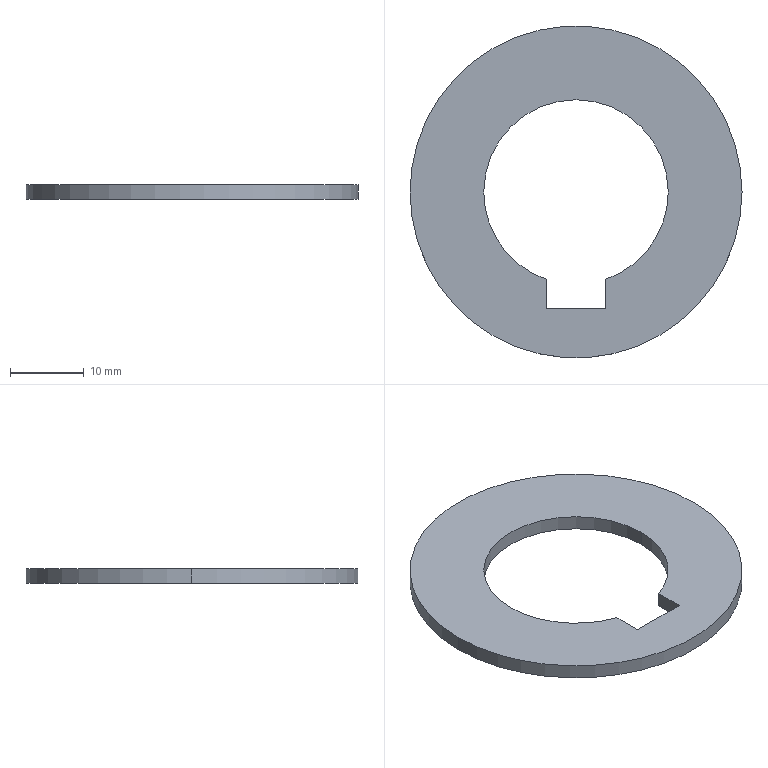Part | NX | 1 solid | 10 faces | box 45 x 45 x 2 mm | volume 2143 mm3 | plane 5 | cylinder 5 | commonest cylinder face diameters 25 x3 45 x2
STEP:
#1=CARTESIAN_POINT('',(-22.5,0.,0.));
#2=VERTEX_POINT('',#1);
#3=CARTESIAN_POINT('',(22.5,0.,0.));
#4=VERTEX_POINT('',#3);
#5=CARTESIAN_POINT('',(0.,0.,0.));
#6=DIRECTION('',(0.,0.,1.));
#7=DIRECTION('',(1.,0.,0.));
#8=AXIS2_PLACEMENT_3D('',#5,#6,#7);
#9=CIRCLE('',#8,22.5);
#10=EDGE_CURVE('',#2,#4,#9,.T.);
#11=ORIENTED_EDGE('',*,*,#10,.F.);
#12=CARTESIAN_POINT('',(0.,0.,0.));
#13=DIRECTION('',(0.,0.,1.));
#14=DIRECTION('',(1.,0.,0.));
#15=AXIS2_PLACEMENT_3D('',#12,#13,#14);
#16=CIRCLE('',#15,22.5);
#17=EDGE_CURVE('',#4,#2,#16,.T.);
#18=ORIENTED_EDGE('',*,*,#17,.F.);
#19=EDGE_LOOP('',(#11,#18));
#20=FACE_BOUND('',#19,.T.);
#21=CARTESIAN_POINT('',(4.,-11.843,0.));
#22=VERTEX_POINT('',#21);
#23=CARTESIAN_POINT('',(12.5,0.,0.));
#24=VERTEX_POINT('',#23);
#25=CARTESIAN_POINT('',(0.,0.,0.));
#26=DIRECTION('',(0.,0.,1.));
#27=DIRECTION('',(-1.,0.,0.));
#28=AXIS2_PLACEMENT_3D('',#25,#26,#27);
#29=CIRCLE('',#28,12.5);
#30=EDGE_CURVE('',#22,#24,#29,.T.);
#31=ORIENTED_EDGE('',*,*,#30,.T.);
#32=CARTESIAN_POINT('',(-12.5,0.,0.));
#33=VERTEX_POINT('',#32);
#34=CARTESIAN_POINT('',(0.,0.,0.));
#35=DIRECTION('',(0.,0.,1.));
#36=DIRECTION('',(-1.,0.,0.));
#37=AXIS2_PLACEMENT_3D('',#34,#35,#36);
#38=CIRCLE('',#37,12.5);
#39=EDGE_CURVE('',#24,#33,#38,.T.);
#40=ORIENTED_EDGE('',*,*,#39,.T.);
#41=CARTESIAN_POINT('',(-4.,-11.843,0.));
#42=VERTEX_POINT('',#41);
#43=CARTESIAN_POINT('',(0.,0.,0.));
#44=DIRECTION('',(0.,0.,1.));
#45=DIRECTION('',(-1.,0.,0.));
#46=AXIS2_PLACEMENT_3D('',#43,#44,#45);
#47=CIRCLE('',#46,12.5);
#48=EDGE_CURVE('',#33,#42,#47,.T.);
#49=ORIENTED_EDGE('',*,*,#48,.T.);
#50=CARTESIAN_POINT('',(-4.,-15.8,0.));
#51=VERTEX_POINT('',#50);
#52=CARTESIAN_POINT('',(-4.,0.,0.));
#53=DIRECTION('',(0.,-1.,0.));
#54=VECTOR('',#53,1000.);
#55=LINE('',#52,#54);
#56=EDGE_CURVE('',#42,#51,#55,.T.);
#57=ORIENTED_EDGE('',*,*,#56,.T.);
#58=CARTESIAN_POINT('',(4.,-15.8,0.));
#59=VERTEX_POINT('',#58);
#60=CARTESIAN_POINT('',(0.,-15.8,0.));
#61=DIRECTION('',(1.,0.,0.));
#62=VECTOR('',#61,1000.);
#63=LINE('',#60,#62);
#64=EDGE_CURVE('',#51,#59,#63,.T.);
#65=ORIENTED_EDGE('',*,*,#64,.T.);
#66=CARTESIAN_POINT('',(4.,0.,0.));
#67=DIRECTION('',(0.,1.,0.));
#68=VECTOR('',#67,1000.);
#69=LINE('',#66,#68);
#70=EDGE_CURVE('',#59,#22,#69,.T.);
#71=ORIENTED_EDGE('',*,*,#70,.T.);
#72=EDGE_LOOP('',(#31,#40,#49,#57,#65,#71));
#73=FACE_BOUND('',#72,.T.);
#74=CARTESIAN_POINT('',(0.,0.,0.));
#75=DIRECTION('',(0.,0.,1.));
#76=DIRECTION('',(1.,0.,0.));
#77=AXIS2_PLACEMENT_3D('',#74,#75,#76);
#78=PLANE('',#77);
#79=ADVANCED_FACE('',(#20,#73),#78,.F.);
#80=CARTESIAN_POINT('',(-22.5,0.,2.));
#81=VERTEX_POINT('',#80);
#82=CARTESIAN_POINT('',(22.5,0.,2.));
#83=VERTEX_POINT('',#82);
#84=CARTESIAN_POINT('',(0.,0.,2.));
#85=DIRECTION('',(0.,0.,1.));
#86=DIRECTION('',(1.,0.,0.));
#87=AXIS2_PLACEMENT_3D('',#84,#85,#86);
#88=CIRCLE('',#87,22.5);
#89=EDGE_CURVE('',#81,#83,#88,.T.);
#90=ORIENTED_EDGE('',*,*,#89,.F.);
#91=CARTESIAN_POINT('',(-22.5,0.,0.));
#92=DIRECTION('',(0.,0.,1.));
#93=VECTOR('',#92,1000.);
#94=LINE('',#91,#93);
#95=EDGE_CURVE('',#2,#81,#94,.T.);
#96=ORIENTED_EDGE('',*,*,#95,.F.);
#97=ORIENTED_EDGE('',*,*,#10,.T.);
#98=CARTESIAN_POINT('',(22.5,0.,0.));
#99=DIRECTION('',(0.,0.,1.));
#100=VECTOR('',#99,1000.);
#101=LINE('',#98,#100);
#102=EDGE_CURVE('',#4,#83,#101,.T.);
#103=ORIENTED_EDGE('',*,*,#102,.T.);
#104=EDGE_LOOP('',(#90,#96,#97,#103));
#105=FACE_BOUND('',#104,.T.);
#106=CARTESIAN_POINT('',(0.,0.,0.));
#107=DIRECTION('',(0.,0.,1.));
#108=DIRECTION('',(1.,0.,0.));
#109=AXIS2_PLACEMENT_3D('',#106,#107,#108);
#110=CYLINDRICAL_SURFACE('',#109,22.5);
#111=ADVANCED_FACE('',(#105),#110,.T.);
#112=ORIENTED_EDGE('',*,*,#89,.T.);
#113=CARTESIAN_POINT('',(0.,0.,2.));
#114=DIRECTION('',(0.,0.,1.));
#115=DIRECTION('',(1.,0.,0.));
#116=AXIS2_PLACEMENT_3D('',#113,#114,#115);
#117=CIRCLE('',#116,22.5);
#118=EDGE_CURVE('',#83,#81,#117,.T.);
#119=ORIENTED_EDGE('',*,*,#118,.T.);
#120=EDGE_LOOP('',(#112,#119));
#121=FACE_BOUND('',#120,.T.);
#122=CARTESIAN_POINT('',(4.,-11.843,2.));
#123=VERTEX_POINT('',#122);
#124=CARTESIAN_POINT('',(12.5,0.,2.));
#125=VERTEX_POINT('',#124);
#126=CARTESIAN_POINT('',(0.,0.,2.));
#127=DIRECTION('',(0.,0.,1.));
#128=DIRECTION('',(-1.,0.,0.));
#129=AXIS2_PLACEMENT_3D('',#126,#127,#128);
#130=CIRCLE('',#129,12.5);
#131=EDGE_CURVE('',#123,#125,#130,.T.);
#132=ORIENTED_EDGE('',*,*,#131,.F.);
#133=CARTESIAN_POINT('',(4.,-15.8,2.));
#134=VERTEX_POINT('',#133);
#135=CARTESIAN_POINT('',(4.,0.,2.));
#136=DIRECTION('',(0.,1.,0.));
#137=VECTOR('',#136,1000.);
#138=LINE('',#135,#137);
#139=EDGE_CURVE('',#134,#123,#138,.T.);
#140=ORIENTED_EDGE('',*,*,#139,.F.);
#141=CARTESIAN_POINT('',(-4.,-15.8,2.));
#142=VERTEX_POINT('',#141);
#143=CARTESIAN_POINT('',(0.,-15.8,2.));
#144=DIRECTION('',(1.,0.,0.));
#145=VECTOR('',#144,1000.);
#146=LINE('',#143,#145);
#147=EDGE_CURVE('',#142,#134,#146,.T.);
#148=ORIENTED_EDGE('',*,*,#147,.F.);
#149=CARTESIAN_POINT('',(-4.,-11.843,2.));
#150=VERTEX_POINT('',#149);
#151=CARTESIAN_POINT('',(-4.,0.,2.));
#152=DIRECTION('',(0.,-1.,0.));
#153=VECTOR('',#152,1000.);
#154=LINE('',#151,#153);
#155=EDGE_CURVE('',#150,#142,#154,.T.);
#156=ORIENTED_EDGE('',*,*,#155,.F.);
#157=CARTESIAN_POINT('',(-12.5,0.,2.));
#158=VERTEX_POINT('',#157);
#159=CARTESIAN_POINT('',(0.,0.,2.));
#160=DIRECTION('',(0.,0.,1.));
#161=DIRECTION('',(-1.,0.,0.));
#162=AXIS2_PLACEMENT_3D('',#159,#160,#161);
#163=CIRCLE('',#162,12.5);
#164=EDGE_CURVE('',#158,#150,#163,.T.);
#165=ORIENTED_EDGE('',*,*,#164,.F.);
#166=CARTESIAN_POINT('',(0.,0.,2.));
#167=DIRECTION('',(0.,0.,1.));
#168=DIRECTION('',(-1.,0.,0.));
#169=AXIS2_PLACEMENT_3D('',#166,#167,#168);
#170=CIRCLE('',#169,12.5);
#171=EDGE_CURVE('',#125,#158,#170,.T.);
#172=ORIENTED_EDGE('',*,*,#171,.F.);
#173=EDGE_LOOP('',(#132,#140,#148,#156,#165,#172));
#174=FACE_BOUND('',#173,.T.);
#175=CARTESIAN_POINT('',(0.,0.,2.));
#176=DIRECTION('',(0.,0.,1.));
#177=DIRECTION('',(1.,0.,0.));
#178=AXIS2_PLACEMENT_3D('',#175,#176,#177);
#179=PLANE('',#178);
#180=ADVANCED_FACE('',(#121,#174),#179,.T.);
#181=CARTESIAN_POINT('',(12.5,0.,-0.2));
#182=DIRECTION('',(0.,0.,1.));
#183=VECTOR('',#182,1000.);
#184=LINE('',#181,#183);
#185=EDGE_CURVE('',#24,#125,#184,.T.);
#186=ORIENTED_EDGE('',*,*,#185,.F.);
#187=ORIENTED_EDGE('',*,*,#30,.F.);
#188=CARTESIAN_POINT('',(4.,-11.843,0.));
#189=DIRECTION('',(0.,0.,1.));
#190=VECTOR('',#189,1000.);
#191=LINE('',#188,#190);
#192=EDGE_CURVE('',#22,#123,#191,.T.);
#193=ORIENTED_EDGE('',*,*,#192,.T.);
#194=ORIENTED_EDGE('',*,*,#131,.T.);
#195=EDGE_LOOP('',(#186,#187,#193,#194));
#196=FACE_BOUND('',#195,.T.);
#197=CARTESIAN_POINT('',(0.,0.,-0.2));
#198=DIRECTION('',(0.,0.,1.));
#199=DIRECTION('',(-1.,0.,0.));
#200=AXIS2_PLACEMENT_3D('',#197,#198,#199);
#201=CYLINDRICAL_SURFACE('',#200,12.5);
#202=ADVANCED_FACE('',(#196),#201,.F.);
#203=ORIENTED_EDGE('',*,*,#64,.F.);
#204=CARTESIAN_POINT('',(-4.,-15.8,-0.2));
#205=DIRECTION('',(0.,0.,1.));
#206=VECTOR('',#205,1000.);
#207=LINE('',#204,#206);
#208=EDGE_CURVE('',#51,#142,#207,.T.);
#209=ORIENTED_EDGE('',*,*,#208,.T.);
#210=ORIENTED_EDGE('',*,*,#147,.T.);
#211=CARTESIAN_POINT('',(4.,-15.8,-0.2));
#212=DIRECTION('',(0.,0.,1.));
#213=VECTOR('',#212,1000.);
#214=LINE('',#211,#213);
#215=EDGE_CURVE('',#59,#134,#214,.T.);
#216=ORIENTED_EDGE('',*,*,#215,.F.);
#217=EDGE_LOOP('',(#203,#209,#210,#216));
#218=FACE_BOUND('',#217,.T.);
#219=CARTESIAN_POINT('',(4.,-15.8,-0.2));
#220=DIRECTION('',(0.,-1.,0.));
#221=DIRECTION('',(0.,0.,-1.));
#222=AXIS2_PLACEMENT_3D('',#219,#220,#221);
#223=PLANE('',#222);
#224=ADVANCED_FACE('',(#218),#223,.F.);
#225=ORIENTED_EDGE('',*,*,#155,.T.);
#226=ORIENTED_EDGE('',*,*,#208,.F.);
#227=ORIENTED_EDGE('',*,*,#56,.F.);
#228=CARTESIAN_POINT('',(-4.,-11.843,0.));
#229=DIRECTION('',(0.,0.,1.));
#230=VECTOR('',#229,1000.);
#231=LINE('',#228,#230);
#232=EDGE_CURVE('',#42,#150,#231,.T.);
#233=ORIENTED_EDGE('',*,*,#232,.T.);
#234=EDGE_LOOP('',(#225,#226,#227,#233));
#235=FACE_BOUND('',#234,.T.);
#236=CARTESIAN_POINT('',(-4.,-15.8,-0.2));
#237=DIRECTION('',(-1.,0.,0.));
#238=DIRECTION('',(0.,0.,1.));
#239=AXIS2_PLACEMENT_3D('',#236,#237,#238);
#240=PLANE('',#239);
#241=ADVANCED_FACE('',(#235),#240,.F.);
#242=ORIENTED_EDGE('',*,*,#139,.T.);
#243=ORIENTED_EDGE('',*,*,#192,.F.);
#244=ORIENTED_EDGE('',*,*,#70,.F.);
#245=ORIENTED_EDGE('',*,*,#215,.T.);
#246=EDGE_LOOP('',(#242,#243,#244,#245));
#247=FACE_BOUND('',#246,.T.);
#248=CARTESIAN_POINT('',(4.,-11.843,-0.2));
#249=DIRECTION('',(1.,0.,0.));
#250=DIRECTION('',(0.,1.,0.));
#251=AXIS2_PLACEMENT_3D('',#248,#249,#250);
#252=PLANE('',#251);
#253=ADVANCED_FACE('',(#247),#252,.F.);
#254=ORIENTED_EDGE('',*,*,#102,.F.);
#255=ORIENTED_EDGE('',*,*,#17,.T.);
#256=ORIENTED_EDGE('',*,*,#95,.T.);
#257=ORIENTED_EDGE('',*,*,#118,.F.);
#258=EDGE_LOOP('',(#254,#255,#256,#257));
#259=FACE_BOUND('',#258,.T.);
#260=CARTESIAN_POINT('',(0.,0.,0.));
#261=DIRECTION('',(0.,0.,1.));
#262=DIRECTION('',(1.,0.,0.));
#263=AXIS2_PLACEMENT_3D('',#260,#261,#262);
#264=CYLINDRICAL_SURFACE('',#263,22.5);
#265=ADVANCED_FACE('',(#259),#264,.T.);
#266=ORIENTED_EDGE('',*,*,#48,.F.);
#267=CARTESIAN_POINT('',(-12.5,0.,-0.2));
#268=DIRECTION('',(0.,0.,1.));
#269=VECTOR('',#268,1000.);
#270=LINE('',#267,#269);
#271=EDGE_CURVE('',#33,#158,#270,.T.);
#272=ORIENTED_EDGE('',*,*,#271,.T.);
#273=ORIENTED_EDGE('',*,*,#164,.T.);
#274=ORIENTED_EDGE('',*,*,#232,.F.);
#275=EDGE_LOOP('',(#266,#272,#273,#274));
#276=FACE_BOUND('',#275,.T.);
#277=CARTESIAN_POINT('',(0.,0.,-0.2));
#278=DIRECTION('',(0.,0.,1.));
#279=DIRECTION('',(-1.,0.,0.));
#280=AXIS2_PLACEMENT_3D('',#277,#278,#279);
#281=CYLINDRICAL_SURFACE('',#280,12.5);
#282=ADVANCED_FACE('',(#276),#281,.F.);
#283=ORIENTED_EDGE('',*,*,#39,.F.);
#284=ORIENTED_EDGE('',*,*,#185,.T.);
#285=ORIENTED_EDGE('',*,*,#171,.T.);
#286=ORIENTED_EDGE('',*,*,#271,.F.);
#287=EDGE_LOOP('',(#283,#284,#285,#286));
#288=FACE_BOUND('',#287,.T.);
#289=CARTESIAN_POINT('',(0.,0.,-0.2));
#290=DIRECTION('',(0.,0.,1.));
#291=DIRECTION('',(-1.,0.,0.));
#292=AXIS2_PLACEMENT_3D('',#289,#290,#291);
#293=CYLINDRICAL_SURFACE('',#292,12.5);
#294=ADVANCED_FACE('',(#288),#293,.F.);
#295=CLOSED_SHELL('',(#79,#111,#180,#202,#224,#241,#253,#265,#282,#294));
#296=MANIFOLD_SOLID_BREP('',#295);
#297=(LENGTH_UNIT()NAMED_UNIT(*)SI_UNIT(.MILLI.,.METRE.));
#298=UNCERTAINTY_MEASURE_WITH_UNIT(LENGTH_MEASURE(0.00001),#297,'','');
#299=(NAMED_UNIT(*)PLANE_ANGLE_UNIT()SI_UNIT($,.RADIAN.));
#300=(NAMED_UNIT(*)SI_UNIT($,.STERADIAN.)SOLID_ANGLE_UNIT());
#301=(GEOMETRIC_REPRESENTATION_CONTEXT(3)GLOBAL_UNCERTAINTY_ASSIGNED_CONTEXT((#298))GLOBAL_UNIT_ASSIGNED_CONTEXT((#297,#299,#300))REPRESENTATION_CONTEXT('',''));
#302=ADVANCED_BREP_SHAPE_REPRESENTATION('',(#296),#301);